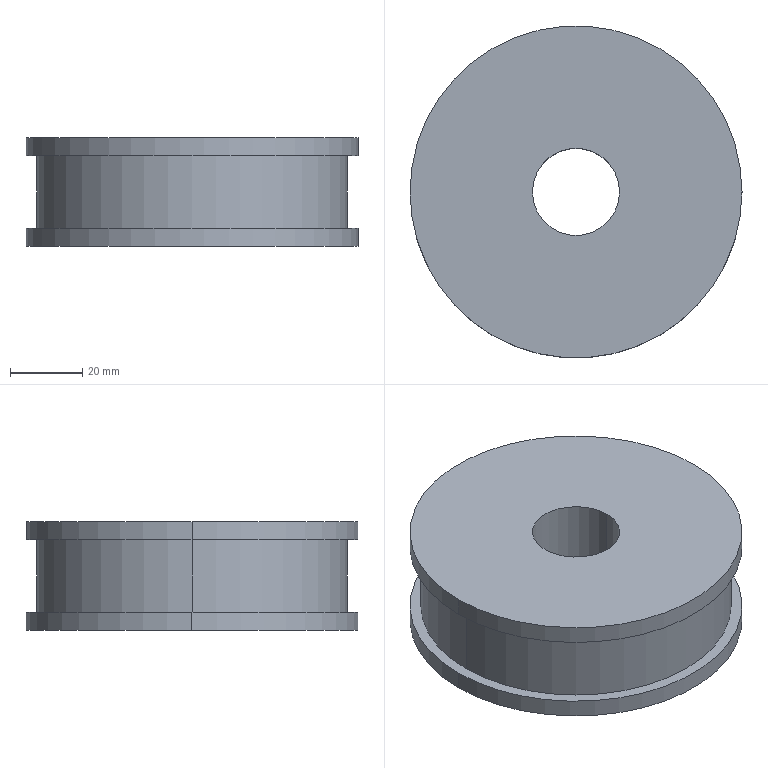Part | SolidWorks | features BaseBody 1 | 1 solid | 12 faces | box 92.189 x 92.189 x 30 mm | volume 169612 mm3 | cylinder 8 | plane 4 | commonest cylinder face diameters 92.189 x4 24.225 x2 86.189 x2
STEP:
#1=CARTESIAN_POINT('',(12.112,0.,25.));
#2=VERTEX_POINT('',#1);
#3=CARTESIAN_POINT('',(-12.112,0.,25.));
#4=VERTEX_POINT('',#3);
#5=CARTESIAN_POINT('',(0.,0.,25.));
#6=DIRECTION('',(0.,0.,-1.));
#7=DIRECTION('',(-1.,0.,0.));
#8=AXIS2_PLACEMENT_3D('',#5,#6,#7);
#9=CIRCLE('',#8,12.112);
#10=EDGE_CURVE('',#2,#4,#9,.T.);
#11=ORIENTED_EDGE('',*,*,#10,.F.);
#12=CARTESIAN_POINT('',(12.112,0.,-5.));
#13=VERTEX_POINT('',#12);
#14=CARTESIAN_POINT('',(12.112,0.,20.));
#15=DIRECTION('',(0.,0.,-1.));
#16=VECTOR('',#15,1000.);
#17=LINE('',#14,#16);
#18=EDGE_CURVE('',#2,#13,#17,.T.);
#19=ORIENTED_EDGE('',*,*,#18,.T.);
#20=CARTESIAN_POINT('',(-12.112,0.,-5.));
#21=VERTEX_POINT('',#20);
#22=CARTESIAN_POINT('',(0.,0.,-5.));
#23=DIRECTION('',(0.,0.,1.));
#24=DIRECTION('',(-1.,0.,0.));
#25=AXIS2_PLACEMENT_3D('',#22,#23,#24);
#26=CIRCLE('',#25,12.112);
#27=EDGE_CURVE('',#21,#13,#26,.T.);
#28=ORIENTED_EDGE('',*,*,#27,.F.);
#29=CARTESIAN_POINT('',(-12.112,0.,20.));
#30=DIRECTION('',(0.,0.,-1.));
#31=VECTOR('',#30,1000.);
#32=LINE('',#29,#31);
#33=EDGE_CURVE('',#4,#21,#32,.T.);
#34=ORIENTED_EDGE('',*,*,#33,.F.);
#35=EDGE_LOOP('',(#11,#19,#28,#34));
#36=FACE_OUTER_BOUND('',#35,.T.);
#37=CARTESIAN_POINT('',(0.,0.,20.));
#38=DIRECTION('',(0.,0.,-1.));
#39=DIRECTION('',(-1.,0.,0.));
#40=AXIS2_PLACEMENT_3D('',#37,#38,#39);
#41=CYLINDRICAL_SURFACE('',#40,12.112);
#42=ADVANCED_FACE('',(#36),#41,.F.);
#43=CARTESIAN_POINT('',(46.095,0.,25.));
#44=VERTEX_POINT('',#43);
#45=CARTESIAN_POINT('',(-46.095,0.,25.));
#46=VERTEX_POINT('',#45);
#47=CARTESIAN_POINT('',(0.,0.,25.));
#48=DIRECTION('',(0.,0.,1.));
#49=DIRECTION('',(-1.,0.,0.));
#50=AXIS2_PLACEMENT_3D('',#47,#48,#49);
#51=CIRCLE('',#50,46.095);
#52=EDGE_CURVE('',#44,#46,#51,.T.);
#53=ORIENTED_EDGE('',*,*,#52,.F.);
#54=CARTESIAN_POINT('',(46.095,0.,20.));
#55=VERTEX_POINT('',#54);
#56=CARTESIAN_POINT('',(46.095,0.,25.));
#57=DIRECTION('',(0.,0.,-1.));
#58=VECTOR('',#57,1000.);
#59=LINE('',#56,#58);
#60=EDGE_CURVE('',#44,#55,#59,.T.);
#61=ORIENTED_EDGE('',*,*,#60,.T.);
#62=CARTESIAN_POINT('',(-46.095,0.,20.));
#63=VERTEX_POINT('',#62);
#64=CARTESIAN_POINT('',(0.,0.,20.));
#65=DIRECTION('',(0.,0.,1.));
#66=DIRECTION('',(-1.,0.,0.));
#67=AXIS2_PLACEMENT_3D('',#64,#65,#66);
#68=CIRCLE('',#67,46.095);
#69=EDGE_CURVE('',#55,#63,#68,.T.);
#70=ORIENTED_EDGE('',*,*,#69,.T.);
#71=CARTESIAN_POINT('',(-46.095,0.,25.));
#72=DIRECTION('',(0.,0.,-1.));
#73=VECTOR('',#72,1000.);
#74=LINE('',#71,#73);
#75=EDGE_CURVE('',#46,#63,#74,.T.);
#76=ORIENTED_EDGE('',*,*,#75,.F.);
#77=EDGE_LOOP('',(#53,#61,#70,#76));
#78=FACE_OUTER_BOUND('',#77,.T.);
#79=CARTESIAN_POINT('',(0.,0.,25.));
#80=DIRECTION('',(0.,0.,-1.));
#81=DIRECTION('',(-1.,0.,0.));
#82=AXIS2_PLACEMENT_3D('',#79,#80,#81);
#83=CYLINDRICAL_SURFACE('',#82,46.095);
#84=ADVANCED_FACE('',(#78),#83,.T.);
#85=CARTESIAN_POINT('',(-46.095,0.,-5.));
#86=VERTEX_POINT('',#85);
#87=CARTESIAN_POINT('',(46.095,0.,-5.));
#88=VERTEX_POINT('',#87);
#89=CARTESIAN_POINT('',(0.,0.,-5.));
#90=DIRECTION('',(0.,0.,-1.));
#91=DIRECTION('',(1.,0.,0.));
#92=AXIS2_PLACEMENT_3D('',#89,#90,#91);
#93=CIRCLE('',#92,46.095);
#94=EDGE_CURVE('',#86,#88,#93,.T.);
#95=ORIENTED_EDGE('',*,*,#94,.F.);
#96=CARTESIAN_POINT('',(-46.095,0.,0.));
#97=VERTEX_POINT('',#96);
#98=CARTESIAN_POINT('',(-46.095,0.,-5.));
#99=DIRECTION('',(0.,0.,1.));
#100=VECTOR('',#99,1000.);
#101=LINE('',#98,#100);
#102=EDGE_CURVE('',#86,#97,#101,.T.);
#103=ORIENTED_EDGE('',*,*,#102,.T.);
#104=CARTESIAN_POINT('',(46.095,0.,0.));
#105=VERTEX_POINT('',#104);
#106=CARTESIAN_POINT('',(0.,0.,0.));
#107=DIRECTION('',(0.,0.,-1.));
#108=DIRECTION('',(1.,0.,0.));
#109=AXIS2_PLACEMENT_3D('',#106,#107,#108);
#110=CIRCLE('',#109,46.095);
#111=EDGE_CURVE('',#97,#105,#110,.T.);
#112=ORIENTED_EDGE('',*,*,#111,.T.);
#113=CARTESIAN_POINT('',(46.095,0.,-5.));
#114=DIRECTION('',(0.,0.,1.));
#115=VECTOR('',#114,1000.);
#116=LINE('',#113,#115);
#117=EDGE_CURVE('',#88,#105,#116,.T.);
#118=ORIENTED_EDGE('',*,*,#117,.F.);
#119=EDGE_LOOP('',(#95,#103,#112,#118));
#120=FACE_OUTER_BOUND('',#119,.T.);
#121=CARTESIAN_POINT('',(0.,0.,-5.));
#122=DIRECTION('',(0.,0.,1.));
#123=DIRECTION('',(1.,0.,0.));
#124=AXIS2_PLACEMENT_3D('',#121,#122,#123);
#125=CYLINDRICAL_SURFACE('',#124,46.095);
#126=ADVANCED_FACE('',(#120),#125,.T.);
#127=CARTESIAN_POINT('',(-43.095,0.,20.));
#128=VERTEX_POINT('',#127);
#129=CARTESIAN_POINT('',(43.095,0.,20.));
#130=VERTEX_POINT('',#129);
#131=CARTESIAN_POINT('',(0.,0.,20.));
#132=DIRECTION('',(0.,0.,-1.));
#133=DIRECTION('',(-1.,0.,0.));
#134=AXIS2_PLACEMENT_3D('',#131,#132,#133);
#135=CIRCLE('',#134,43.095);
#136=EDGE_CURVE('',#128,#130,#135,.T.);
#137=ORIENTED_EDGE('',*,*,#136,.T.);
#138=CARTESIAN_POINT('',(43.095,0.,0.));
#139=VERTEX_POINT('',#138);
#140=CARTESIAN_POINT('',(43.095,0.,20.));
#141=DIRECTION('',(0.,0.,-1.));
#142=VECTOR('',#141,1000.);
#143=LINE('',#140,#142);
#144=EDGE_CURVE('',#130,#139,#143,.T.);
#145=ORIENTED_EDGE('',*,*,#144,.T.);
#146=CARTESIAN_POINT('',(-43.095,0.,0.));
#147=VERTEX_POINT('',#146);
#148=CARTESIAN_POINT('',(0.,0.,0.));
#149=DIRECTION('',(0.,0.,1.));
#150=DIRECTION('',(-1.,0.,0.));
#151=AXIS2_PLACEMENT_3D('',#148,#149,#150);
#152=CIRCLE('',#151,43.095);
#153=EDGE_CURVE('',#139,#147,#152,.T.);
#154=ORIENTED_EDGE('',*,*,#153,.T.);
#155=CARTESIAN_POINT('',(-43.095,0.,20.));
#156=DIRECTION('',(0.,0.,-1.));
#157=VECTOR('',#156,1000.);
#158=LINE('',#155,#157);
#159=EDGE_CURVE('',#128,#147,#158,.T.);
#160=ORIENTED_EDGE('',*,*,#159,.F.);
#161=EDGE_LOOP('',(#137,#145,#154,#160));
#162=FACE_OUTER_BOUND('',#161,.T.);
#163=CARTESIAN_POINT('',(0.,0.,20.));
#164=DIRECTION('',(0.,0.,-1.));
#165=DIRECTION('',(-1.,0.,0.));
#166=AXIS2_PLACEMENT_3D('',#163,#164,#165);
#167=CYLINDRICAL_SURFACE('',#166,43.095);
#168=ADVANCED_FACE('',(#162),#167,.T.);
#169=CARTESIAN_POINT('',(0.,0.,25.));
#170=DIRECTION('',(0.,0.,-1.));
#171=DIRECTION('',(-1.,0.,0.));
#172=AXIS2_PLACEMENT_3D('',#169,#170,#171);
#173=CIRCLE('',#172,12.112);
#174=EDGE_CURVE('',#4,#2,#173,.T.);
#175=ORIENTED_EDGE('',*,*,#174,.T.);
#176=ORIENTED_EDGE('',*,*,#10,.T.);
#177=EDGE_LOOP('',(#175,#176));
#178=FACE_BOUND('',#177,.T.);
#179=CARTESIAN_POINT('',(0.,0.,25.));
#180=DIRECTION('',(0.,0.,1.));
#181=DIRECTION('',(-1.,0.,0.));
#182=AXIS2_PLACEMENT_3D('',#179,#180,#181);
#183=CIRCLE('',#182,46.095);
#184=EDGE_CURVE('',#46,#44,#183,.T.);
#185=ORIENTED_EDGE('',*,*,#184,.T.);
#186=ORIENTED_EDGE('',*,*,#52,.T.);
#187=EDGE_LOOP('',(#185,#186));
#188=FACE_OUTER_BOUND('',#187,.T.);
#189=CARTESIAN_POINT('',(0.,0.,25.));
#190=DIRECTION('',(0.,0.,1.));
#191=DIRECTION('',(1.,0.,0.));
#192=AXIS2_PLACEMENT_3D('',#189,#190,#191);
#193=PLANE('',#192);
#194=ADVANCED_FACE('',(#178,#188),#193,.T.);
#195=ORIENTED_EDGE('',*,*,#18,.F.);
#196=ORIENTED_EDGE('',*,*,#174,.F.);
#197=ORIENTED_EDGE('',*,*,#33,.T.);
#198=CARTESIAN_POINT('',(0.,0.,-5.));
#199=DIRECTION('',(0.,0.,1.));
#200=DIRECTION('',(-1.,0.,0.));
#201=AXIS2_PLACEMENT_3D('',#198,#199,#200);
#202=CIRCLE('',#201,12.112);
#203=EDGE_CURVE('',#13,#21,#202,.T.);
#204=ORIENTED_EDGE('',*,*,#203,.F.);
#205=EDGE_LOOP('',(#195,#196,#197,#204));
#206=FACE_OUTER_BOUND('',#205,.T.);
#207=CARTESIAN_POINT('',(0.,0.,20.));
#208=DIRECTION('',(0.,0.,-1.));
#209=DIRECTION('',(-1.,0.,0.));
#210=AXIS2_PLACEMENT_3D('',#207,#208,#209);
#211=CYLINDRICAL_SURFACE('',#210,12.112);
#212=ADVANCED_FACE('',(#206),#211,.F.);
#213=ORIENTED_EDGE('',*,*,#60,.F.);
#214=ORIENTED_EDGE('',*,*,#184,.F.);
#215=ORIENTED_EDGE('',*,*,#75,.T.);
#216=CARTESIAN_POINT('',(0.,0.,20.));
#217=DIRECTION('',(0.,0.,1.));
#218=DIRECTION('',(-1.,0.,0.));
#219=AXIS2_PLACEMENT_3D('',#216,#217,#218);
#220=CIRCLE('',#219,46.095);
#221=EDGE_CURVE('',#63,#55,#220,.T.);
#222=ORIENTED_EDGE('',*,*,#221,.T.);
#223=EDGE_LOOP('',(#213,#214,#215,#222));
#224=FACE_OUTER_BOUND('',#223,.T.);
#225=CARTESIAN_POINT('',(0.,0.,25.));
#226=DIRECTION('',(0.,0.,-1.));
#227=DIRECTION('',(-1.,0.,0.));
#228=AXIS2_PLACEMENT_3D('',#225,#226,#227);
#229=CYLINDRICAL_SURFACE('',#228,46.095);
#230=ADVANCED_FACE('',(#224),#229,.T.);
#231=ORIENTED_EDGE('',*,*,#27,.T.);
#232=ORIENTED_EDGE('',*,*,#203,.T.);
#233=EDGE_LOOP('',(#231,#232));
#234=FACE_BOUND('',#233,.T.);
#235=CARTESIAN_POINT('',(0.,0.,-5.));
#236=DIRECTION('',(0.,0.,-1.));
#237=DIRECTION('',(1.,0.,0.));
#238=AXIS2_PLACEMENT_3D('',#235,#236,#237);
#239=CIRCLE('',#238,46.095);
#240=EDGE_CURVE('',#88,#86,#239,.T.);
#241=ORIENTED_EDGE('',*,*,#240,.T.);
#242=ORIENTED_EDGE('',*,*,#94,.T.);
#243=EDGE_LOOP('',(#241,#242));
#244=FACE_OUTER_BOUND('',#243,.T.);
#245=CARTESIAN_POINT('',(0.,0.,-5.));
#246=DIRECTION('',(0.,0.,-1.));
#247=DIRECTION('',(-1.,0.,0.));
#248=AXIS2_PLACEMENT_3D('',#245,#246,#247);
#249=PLANE('',#248);
#250=ADVANCED_FACE('',(#234,#244),#249,.T.);
#251=ORIENTED_EDGE('',*,*,#136,.F.);
#252=CARTESIAN_POINT('',(0.,0.,20.));
#253=DIRECTION('',(0.,0.,-1.));
#254=DIRECTION('',(-1.,0.,0.));
#255=AXIS2_PLACEMENT_3D('',#252,#253,#254);
#256=CIRCLE('',#255,43.095);
#257=EDGE_CURVE('',#130,#128,#256,.T.);
#258=ORIENTED_EDGE('',*,*,#257,.F.);
#259=EDGE_LOOP('',(#251,#258));
#260=FACE_BOUND('',#259,.T.);
#261=ORIENTED_EDGE('',*,*,#221,.F.);
#262=ORIENTED_EDGE('',*,*,#69,.F.);
#263=EDGE_LOOP('',(#261,#262));
#264=FACE_OUTER_BOUND('',#263,.T.);
#265=CARTESIAN_POINT('',(0.,0.,20.));
#266=DIRECTION('',(0.,0.,1.));
#267=DIRECTION('',(1.,0.,0.));
#268=AXIS2_PLACEMENT_3D('',#265,#266,#267);
#269=PLANE('',#268);
#270=ADVANCED_FACE('',(#260,#264),#269,.F.);
#271=ORIENTED_EDGE('',*,*,#102,.F.);
#272=ORIENTED_EDGE('',*,*,#240,.F.);
#273=ORIENTED_EDGE('',*,*,#117,.T.);
#274=CARTESIAN_POINT('',(0.,0.,0.));
#275=DIRECTION('',(0.,0.,-1.));
#276=DIRECTION('',(1.,0.,0.));
#277=AXIS2_PLACEMENT_3D('',#274,#275,#276);
#278=CIRCLE('',#277,46.095);
#279=EDGE_CURVE('',#105,#97,#278,.T.);
#280=ORIENTED_EDGE('',*,*,#279,.T.);
#281=EDGE_LOOP('',(#271,#272,#273,#280));
#282=FACE_OUTER_BOUND('',#281,.T.);
#283=CARTESIAN_POINT('',(0.,0.,-5.));
#284=DIRECTION('',(0.,0.,1.));
#285=DIRECTION('',(1.,0.,0.));
#286=AXIS2_PLACEMENT_3D('',#283,#284,#285);
#287=CYLINDRICAL_SURFACE('',#286,46.095);
#288=ADVANCED_FACE('',(#282),#287,.T.);
#289=ORIENTED_EDGE('',*,*,#144,.F.);
#290=ORIENTED_EDGE('',*,*,#257,.T.);
#291=ORIENTED_EDGE('',*,*,#159,.T.);
#292=CARTESIAN_POINT('',(0.,0.,0.));
#293=DIRECTION('',(0.,0.,1.));
#294=DIRECTION('',(-1.,0.,0.));
#295=AXIS2_PLACEMENT_3D('',#292,#293,#294);
#296=CIRCLE('',#295,43.095);
#297=EDGE_CURVE('',#147,#139,#296,.T.);
#298=ORIENTED_EDGE('',*,*,#297,.T.);
#299=EDGE_LOOP('',(#289,#290,#291,#298));
#300=FACE_OUTER_BOUND('',#299,.T.);
#301=CARTESIAN_POINT('',(0.,0.,20.));
#302=DIRECTION('',(0.,0.,-1.));
#303=DIRECTION('',(-1.,0.,0.));
#304=AXIS2_PLACEMENT_3D('',#301,#302,#303);
#305=CYLINDRICAL_SURFACE('',#304,43.095);
#306=ADVANCED_FACE('',(#300),#305,.T.);
#307=ORIENTED_EDGE('',*,*,#297,.F.);
#308=ORIENTED_EDGE('',*,*,#153,.F.);
#309=EDGE_LOOP('',(#307,#308));
#310=FACE_BOUND('',#309,.T.);
#311=ORIENTED_EDGE('',*,*,#279,.F.);
#312=ORIENTED_EDGE('',*,*,#111,.F.);
#313=EDGE_LOOP('',(#311,#312));
#314=FACE_OUTER_BOUND('',#313,.T.);
#315=CARTESIAN_POINT('',(0.,0.,0.));
#316=DIRECTION('',(0.,0.,-1.));
#317=DIRECTION('',(-1.,0.,0.));
#318=AXIS2_PLACEMENT_3D('',#315,#316,#317);
#319=PLANE('',#318);
#320=ADVANCED_FACE('',(#310,#314),#319,.F.);
#321=CLOSED_SHELL('',(#42,#84,#126,#168,#194,#212,#230,#250,#270,#288,#306,#320));
#322=MANIFOLD_SOLID_BREP('',#321);
#323=CARTESIAN_POINT('',(0.,0.,0.));
#324=DIRECTION('',(0.,0.,1.));
#325=DIRECTION('',(1.,0.,0.));
#326=AXIS2_PLACEMENT_3D('',#323,#324,#325);
#327=(LENGTH_UNIT()NAMED_UNIT(*)SI_UNIT(.MILLI.,.METRE.));
#328=UNCERTAINTY_MEASURE_WITH_UNIT(LENGTH_MEASURE(0.00001),#327,'','');
#329=(NAMED_UNIT(*)PLANE_ANGLE_UNIT()SI_UNIT($,.RADIAN.));
#330=(NAMED_UNIT(*)SI_UNIT($,.STERADIAN.)SOLID_ANGLE_UNIT());
#331=(GEOMETRIC_REPRESENTATION_CONTEXT(3)GLOBAL_UNCERTAINTY_ASSIGNED_CONTEXT((#328))GLOBAL_UNIT_ASSIGNED_CONTEXT((#327,#329,#330))REPRESENTATION_CONTEXT('',''));
#332=ADVANCED_BREP_SHAPE_REPRESENTATION('',(#322,#326),#331);